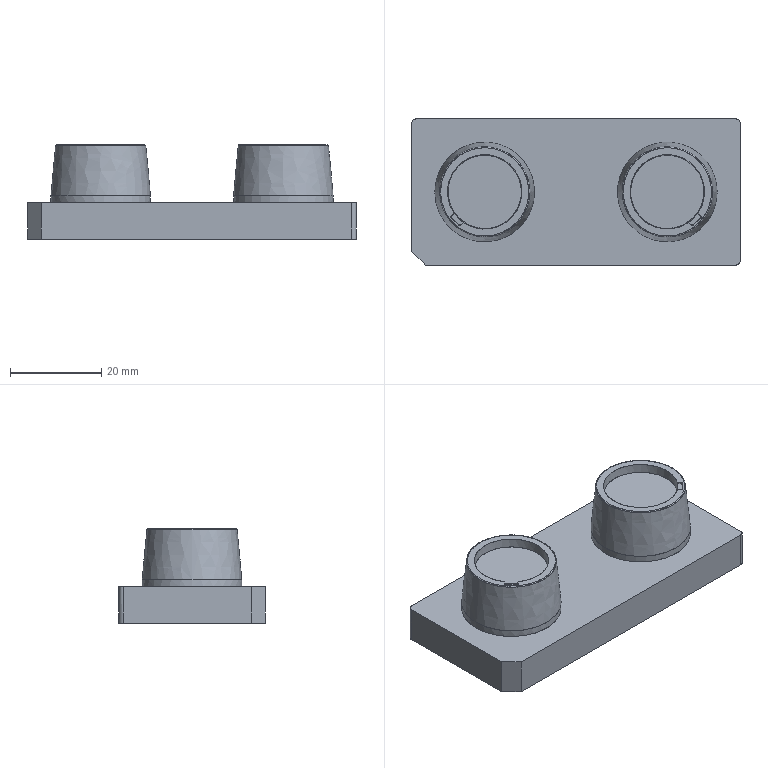NC program | PowerMill | posted with a generic post | part box 72 x 32 x 20.655 mm
Lines 1 to 915 of 315359:
%
O0001
N104 ( POWERMILL CB  : 2026004.0)
N105 ( POST VER      : 2026.0.0.5161)
N106 ( OPTION FILE   : FANUC)
N107 ( OUTPUT WORKPLANE : WORLD)
N108 (  )
N109 ( TOOL LIST )
N110 (---------------------------------------)
N111 ( NO. | ID        | DIA.| TIP RAD|LENGTH)
N112 (---------------------------------------)
N113 (    1|D10C_1_1_1 |10.0 |  0.0   |76.12 )
N114 (    2|D4C_1_1    | 4.0 |  0.0   |67.84 )
N115 (    3|D10_1_1_1  |10.0 |  0.0   | 75.8 )
N116 (    5|B4R0.5_1_1 | 4.0 |  0.5   | 67.8 )
N117 (    8|D1_1       | 1.0 |  0.0   | 56.0 )
N118 (   13|TEXT_D4_1_1| 4.0 |  0.3   |67.92 )
N119 (---------------------------------------)
N120 (  )
N121 ( NUMBER OF TOOLPATHS: 13.0 )
N122 ( ESTIMATED PROGRAM DURATION: 0 HOURS 36 MIN 15 SEC)
N123 (  )
N124 G00 G21 G80 G40 G17
N125 G90
N126 G54
N127 G53 Z0.0
N128 (---------------)
N129 ( START TOOLPATH : 精公开粗01-扫面平行-D10C )
N130 (---------------)
N131 ( TOOL NO.    :1 )
N132 ( TOOL TYPE   : ENDMILL)
N133 ( TOOL ID     : D10C_1_1_1)
N134 ( TOOL DIA    : 10.0 LENGTH 76.12)
N135 T1
N136 M6
N137 S8000 M03
N138 G00 G90 X0.0 Y0.0
N139 G43 Z10.2 H1
N140
N141 G05 P10000 R4
N142 X43.78 Y18.78
N143 Z1.135
N144 G01 Z-0.065 F6000.0
N145 X38.78 F10000.0
N146 X-38.78
N147 Y13.4143
N148 X38.78
N149 Y8.0486
N150 X-38.78
N151 Y2.6829
N152 X38.78
N153 Y-2.6829
N154 X-38.78
N155 Y-8.0486
N156 X38.78
N157 Y-13.4143
N158 X-38.78
N159 Y-18.78
N160 X38.78
N161 X43.78
N162 G00 Z10.2
N163 G05 P0
N164 (---------------)
N165 ( END TOOLPATH : 精公开粗01-扫面平行-D10C )
N166 (---------------)
N167 ( START TOOLPATH : 精公开粗01-外形偏置-D10C )
N168 (---------------)
N169 G00 X0.0 Y0.0 Z9.885
N170 G05 P10000 R4
N171 X19.903 Y-2.8285
N172 Z1.1899
N173 G01 Z-0.0101 F6000.0
N174 X20.1091 Y-2.8335 Z-0.0137
N175 X20.501 Y-2.7901 Z-0.0206
N176 X20.8825 Y-2.6933 Z-0.0274
N177 X21.2741 Y-2.5346 Z-0.0348
N178 X21.6402 Y-2.3203 Z-0.0422
N179 X21.9587 Y-2.1244 Z-0.0488
N180 X22.123 Y-1.96 Z-0.0528
N181 X22.4294 Y-1.4606 Z-0.063
N182 X22.6008 Y-1.1271 Z-0.0696
N183 X22.7288 Y-0.7734 Z-0.0761
N184 X22.8112 Y-0.3909 Z-0.083
N185 X22.835 Y0.0 Z-0.0898
N186 X22.8067 Y0.3906 Z-0.0966
N187 X22.726 Y0.7734 Z-0.1035
N188 X22.6003 Y1.1275 Z-0.11
N189 X22.4294 Y1.4635 Z-0.1166
N190 X22.2257 Y1.76 Z-0.1229
N191 X22.0503 Y1.9572 Z-0.1275
N192 X21.6237 Y2.3203 Z-0.1373
N193 X21.2669 Y2.5338 Z-0.1445
N194 X20.8825 Y2.695 Z-0.1518
N195 X20.5011 Y2.791 Z-0.1587
N196 X20.1091 Y2.8316 Z-0.1655
N197 X19.7195 Y2.8187 Z-0.1723
N198 X19.3357 Y2.7535 Z-0.1791
N199 X18.9368 Y2.6276 Z-0.1864
N200 X18.5622 Y2.4457 Z-0.1937
N201 X18.3116 Y2.2576 Z-0.1992
N202 X18.061 Y2.0696 Z-0.2046
N203 X17.9212 Y1.9247 Z-0.2081
N204 X17.6227 Y1.5469 Z-0.2166
N205 X17.4192 Y1.1743 Z-0.224
N206 X17.2744 Y0.7734 Z-0.2314
N207 X17.1936 Y0.3907 Z-0.2382
N208 X17.1655 Y0.0 Z-0.2451
N209 X17.1902 Y-0.3908 Z-0.2519
N210 X17.27 Y-0.7734 Z-0.2587
N211 X17.4201 Y-1.1736 Z-0.2662
N212 X17.6254 Y-1.5469 Z-0.2736
N213 X17.7888 Y-1.7726 Z-0.2785
N214 X18.0606 Y-2.0667 Z-0.2855
N215 X18.3701 Y-2.3203 Z-0.2924
N216 X18.5622 Y-2.4423 Z-0.2964
N217 X18.9369 Y-2.6281 Z-0.3037
N218 X19.3357 Y-2.7581 Z-0.311
N219 X19.7193 Y-2.824 Z-0.3178
N220 X20.1091 Y-2.8335 Z-0.3246
N221 X20.501 Y-2.7901 Z-0.3315
N222 X20.8825 Y-2.6933 Z-0.3384
N223 X21.2741 Y-2.5346 Z-0.3458
N224 X21.6402 Y-2.3203 Z-0.3532
N225 X21.9587 Y-2.1244 Z-0.3597
N226 X22.123 Y-1.96 Z-0.3637
N227 X22.4294 Y-1.4606 Z-0.374
N228 X22.6008 Y-1.1271 Z-0.3805
N229 X22.7288 Y-0.7734 Z-0.3871
N230 X22.8112 Y-0.3909 Z-0.3939
N231 X22.835 Y0.0 Z-0.4007
N232 X22.8067 Y0.3906 Z-0.4076
N233 X22.726 Y0.7734 Z-0.4144
N234 X22.6003 Y1.1275 Z-0.421
N235 X22.4294 Y1.4635 Z-0.4275
N236 X22.2257 Y1.76 Z-0.4338
N237 X22.0503 Y1.9572 Z-0.4384
N238 X21.6237 Y2.3203 Z-0.4482
N239 X21.2669 Y2.5338 Z-0.4555
N240 X20.8825 Y2.695 Z-0.4627
N241 X20.5011 Y2.791 Z-0.4696
N242 X20.1091 Y2.8316 Z-0.4765
N243 X19.7195 Y2.8187 Z-0.4833
N244 X19.3357 Y2.7535 Z-0.4901
N245 X18.9368 Y2.6276 Z-0.4974
N246 X18.5622 Y2.4457 Z-0.5046
N247 X18.3116 Y2.2576 Z-0.5101
N248 X18.061 Y2.0696 F10000.0
N249 X17.9212 Y1.9247
N250 X17.6227 Y1.5469
N251 X17.4192 Y1.1743
N252 X17.2744 Y0.7734
N253 X17.1936 Y0.3907
N254 X17.1655 Y0.0
N255 X17.1902 Y-0.3908
N256 X17.27 Y-0.7734
N257 X17.4201 Y-1.1736
N258 X17.6254 Y-1.5469
N259 X17.7888 Y-1.7726
N260 X18.0606 Y-2.0667
N261 X18.3701 Y-2.3203
N262 X18.5622 Y-2.4423
N263 X18.9369 Y-2.6281
N264 X19.3357 Y-2.7581
N265 X19.7193 Y-2.824
N266 X20.1091 Y-2.8335
N267 X20.501 Y-2.7901
N268 X20.8825 Y-2.6933
N269 X21.2741 Y-2.5346
N270 X21.6402 Y-2.3203
N271 X21.9587 Y-2.1244
N272 X22.0505 Y-2.0518
N273 X22.123 Y-1.96
N274 X22.4294 Y-1.4606
N275 X22.6008 Y-1.1271
N276 X22.7288 Y-0.7734
N277 X22.8112 Y-0.3909
N278 X22.835 Y0.0
N279 X22.8067 Y0.3906
N280 X22.726 Y0.7734
N281 X22.6003 Y1.1275
N282 X22.4294 Y1.4635
N283 X22.2257 Y1.76
N284 X22.0503 Y1.9572
N285 X21.6237 Y2.3203
N286 X21.2669 Y2.5338
N287 X20.8825 Y2.695
N288 X20.5011 Y2.791
N289 X20.1091 Y2.8316
N290 X19.7195 Y2.8187
N291 X19.3357 Y2.7535
N292 X18.9368 Y2.6276
N293 X18.5622 Y2.4457
N294 X18.3116 Y2.2576
N295 G00 Z5.843
N296 G01 X19.6442 Y-2.7896
N297 G00 Z-0.4052
N298 G01 X19.7191 Y-2.8028 Z-0.4065 F6000.0
N299 X20.1091 Y-2.8122 Z-0.4133
N300 X20.6953 Y-2.7282 Z-0.4237
N301 X21.251 Y-2.5191 Z-0.434
N302 X21.5966 Y-2.3203 Z-0.441
N303 X22.009 Y-1.9677 Z-0.4505
N304 X22.352 Y-1.5469 Z-0.4599
N305 X22.5869 Y-1.106 Z-0.4687
N306 X22.7066 Y-0.7734 Z-0.4748
N307 X22.7887 Y-0.3907 Z-0.4816
N308 X22.814 Y0.0 Z-0.4885
N309 X22.7858 Y0.3907 Z-0.4953
N310 X22.7044 Y0.7734 Z-0.5021
N311 X22.5869 Y1.1047 Z-0.5083
N312 X22.4294 Y1.4201 Z-0.5144
N313 X22.0357 Y1.9425 Z-0.5259
N314 X21.6559 Y2.2728 Z-0.5346
N315 X21.2477 Y2.5206 Z-0.543
N316 X20.8825 Y2.6728 Z-0.5499
N317 X20.5012 Y2.7702 Z-0.5567
N318 X20.1091 Y2.8113 Z-0.5636
N319 X19.7195 Y2.7979 Z-0.5704
N320 X19.3357 Y2.7321 Z-0.5772
N321 X18.9367 Y2.6046 Z-0.5845
N322 X18.5622 Y2.4207 Z-0.5918
N323 X18.3242 Y2.241 Z-0.597
N324 X18.0773 Y2.0546 Z-0.6024
N325 X17.9275 Y1.901 Z-0.6062
N326 X17.6489 Y1.5469 Z-0.614
N327 X17.4419 Y1.1751 Z-0.6214
N328 X17.2632 Y0.6374 Z-0.6313
N329 X17.2403 Y0.5302 Z-0.6333
N330 X17.1865 Y0.0 Z-0.6426
N331 X17.213 Y-0.3905 Z-0.6494
N332 X17.2921 Y-0.7734 Z-0.6562
N333 X17.4432 Y-1.174 Z-0.6637
N334 X17.6503 Y-1.5469 Z-0.6711
N335 X17.9254 Y-1.9026 Z-0.679
N336 X18.4084 Y-2.3203 Z-0.6901
N337 X18.7437 Y-2.5205 Z-0.6969
N338 X19.3357 Y-2.7349 Z-0.7079
N339 X19.7191 Y-2.8028 Z-0.7147
N340 X20.1091 Y-2.8122 Z-0.7215
N341 X20.6953 Y-2.7282 Z-0.7319
N342 X21.251 Y-2.5191 Z-0.7422
N343 X21.5966 Y-2.3203 Z-0.7492
N344 X22.009 Y-1.9677 Z-0.7586
N345 X22.352 Y-1.5469 Z-0.7681
N346 X22.5869 Y-1.106 Z-0.7768
N347 X22.7066 Y-0.7734 Z-0.783
N348 X22.7887 Y-0.3907 Z-0.7898
N349 X22.814 Y0.0 Z-0.7967
N350 X22.7858 Y0.3907 Z-0.8035
N351 X22.7044 Y0.7734 Z-0.8103
N352 X22.5869 Y1.1047 Z-0.8165
N353 X22.4294 Y1.4201 Z-0.8226
N354 X22.0357 Y1.9425 Z-0.834
N355 X21.6559 Y2.2728 Z-0.8428
N356 X21.2477 Y2.5206 Z-0.8512
N357 X20.8825 Y2.6728 Z-0.8581
N358 X20.5012 Y2.7702 Z-0.8649
N359 X20.1091 Y2.8113 Z-0.8718
N360 X19.7195 Y2.7979 Z-0.8786
N361 X19.3357 Y2.7321 Z-0.8854
N362 X18.9367 Y2.6046 Z-0.8927
N363 X18.5622 Y2.4207 Z-0.9
N364 X18.3242 Y2.241 Z-0.9052
N365 X18.0773 Y2.0546 F10000.0
N366 X17.9275 Y1.901
N367 X17.6489 Y1.5469
N368 X17.4419 Y1.1751
N369 X17.2632 Y0.6374
N370 X17.2488 Y0.5844
N371 X17.2403 Y0.5302
N372 X17.1865 Y0.0
N373 X17.213 Y-0.3905
N374 X17.2921 Y-0.7734
N375 X17.4432 Y-1.174
N376 X17.6503 Y-1.5469
N377 X17.9254 Y-1.9026
N378 X18.4084 Y-2.3203
N379 X18.7437 Y-2.5205
N380 X19.3357 Y-2.7349
N381 X19.7191 Y-2.8028
N382 X20.1091 Y-2.8122
N383 X20.6953 Y-2.7282
N384 X21.251 Y-2.5191
N385 X21.5966 Y-2.3203
N386 X22.009 Y-1.9677
N387 X22.352 Y-1.5469
N388 X22.5869 Y-1.106
N389 X22.7066 Y-0.7734
N390 X22.7887 Y-0.3907
N391 X22.814 Y0.0
N392 X22.7858 Y0.3907
N393 X22.7044 Y0.7734
N394 X22.5869 Y1.1047
N395 X22.4294 Y1.4201
N396 X22.0357 Y1.9425
N397 X21.6559 Y2.2728
N398 X21.2477 Y2.5206
N399 X20.8825 Y2.6728
N400 X20.5012 Y2.7702
N401 X20.1091 Y2.8113
N402 X19.7195 Y2.7979
N403 X19.3357 Y2.7321
N404 X18.9367 Y2.6046
N405 X18.5622 Y2.4207
N406 X18.3242 Y2.241
N407 G00 Z5.8378
N408 G01 X19.4393 Y-2.7343
N409 G00 Z-0.8003
N410 G01 X19.7204 Y-2.782 Z-0.8053 F6000.0
N411 X20.1091 Y-2.7908 Z-0.8121
N412 X20.5009 Y-2.7455 Z-0.8189
N413 X20.8825 Y-2.6474 Z-0.8258
N414 X21.2287 Y-2.5062 Z-0.8323
N415 X21.2573 Y-2.4898 Z-0.8329
N416 X21.5538 Y-2.3203 Z-0.8389
N417 X22.0217 Y-1.9256 Z-0.8496
N418 X22.3257 Y-1.5469 Z-0.858
N419 X22.5755 Y-1.0858 Z-0.8672
N420 X22.6843 Y-0.7734 Z-0.873
N421 X22.7692 Y-0.3911 Z-0.8798
N422 X22.7931 Y0.0 Z-0.8866
N423 X22.7639 Y0.3906 Z-0.8935
N424 X22.6828 Y0.7734 Z-0.9003
N425 X22.5737 Y1.0817 Z-0.906
N426 X22.3252 Y1.5469 Z-0.9152
N427 X22.0211 Y1.9278 Z-0.9237
N428 X21.6559 Y2.2476 Z-0.9322
N429 X21.2283 Y2.5071 Z-0.9409
N430 X20.8825 Y2.6506 Z-0.9475
N431 X20.5012 Y2.7493 Z-0.9543
N432 X20.1091 Y2.791 Z-0.9612
N433 X19.7195 Y2.7765 Z-0.968
N434 X19.3357 Y2.7107 Z-0.9748
N435 X18.9355 Y2.5843 Z-0.9821
N436 X18.5622 Y2.3957 Z-0.9894
N437 X18.3364 Y2.2248 Z-0.9944
N438 X18.0927 Y2.0405 Z-0.9997
N439 X17.6723 Y1.5469 Z-1.011
N440 X17.4644 Y1.175 Z-1.0185
N441 X17.3181 Y0.7734 Z-1.0259
N442 X17.2366 Y0.391 Z-1.0327
N443 X17.207 Y0.0 Z-1.0396
N444 X17.2308 Y-0.3908 Z-1.0464
N445 X17.3141 Y-0.7734 Z-1.0532
N446 X17.4676 Y-1.173 Z-1.0607
N447 X17.6756 Y-1.5469 Z-1.0682
N448 X17.7888 Y-1.7051 Z-1.0716
N449 X18.0926 Y-2.0376 Z-1.0794
N450 X18.4434 Y-2.3203 Z-1.0873
N451 X18.9388 Y-2.5811 Z-1.0971
N452 X19.3357 Y-2.7167 Z-1.1044
N453 X19.7204 Y-2.782 Z-1.1112
N454 X20.1091 Y-2.7908 Z-1.118
N455 X20.5009 Y-2.7455 Z-1.1249
N456 X20.8825 Y-2.6474 Z-1.1317
N457 X21.2287 Y-2.5062 Z-1.1383
N458 X21.2573 Y-2.4898 Z-1.1388
N459 X21.5538 Y-2.3203 Z-1.1448
N460 X22.0217 Y-1.9256 Z-1.1555
N461 X22.3257 Y-1.5469 Z-1.164
N462 X22.5755 Y-1.0858 Z-1.1731
N463 X22.6843 Y-0.7734 Z-1.1789
N464 X22.7692 Y-0.3911 Z-1.1857
N465 X22.7931 Y0.0 Z-1.1926
N466 X22.7639 Y0.3906 Z-1.1994
N467 X22.6828 Y0.7734 Z-1.2062
N468 X22.5737 Y1.0817 Z-1.2119
N469 X22.3252 Y1.5469 Z-1.2211
N470 X22.0211 Y1.9278 Z-1.2296
N471 X21.6559 Y2.2476 Z-1.2381
N472 X21.2283 Y2.5071 Z-1.2468
N473 X20.8825 Y2.6506 Z-1.2534
N474 X20.5012 Y2.7493 Z-1.2603
N475 X20.1091 Y2.791 Z-1.2671
N476 X19.7195 Y2.7765 Z-1.2739
N477 X19.3357 Y2.7107 Z-1.2807
N478 X18.9355 Y2.5843 Z-1.2881
N479 X18.5622 Y2.3957 Z-1.2954
N480 X18.3364 Y2.2248 Z-1.3003
N481 X18.0927 Y2.0405 F10000.0
N482 X17.6723 Y1.5469
N483 X17.4644 Y1.175
N484 X17.3181 Y0.7734
N485 X17.2366 Y0.391
N486 X17.207 Y0.0
N487 X17.2308 Y-0.3908
N488 X17.3141 Y-0.7734
N489 X17.4676 Y-1.173
N490 X17.6756 Y-1.5469
N491 X17.7888 Y-1.7051
N492 X18.0926 Y-2.0376
N493 X18.4434 Y-2.3203
N494 X18.9388 Y-2.5811
N495 X19.3357 Y-2.7167
N496 X19.7204 Y-2.782
N497 X20.1091 Y-2.7908
N498 X20.5009 Y-2.7455
N499 X20.8825 Y-2.6474
N500 X21.2287 Y-2.5062
N501 X21.2573 Y-2.4898
N502 X21.5538 Y-2.3203
N503 X22.0217 Y-1.9256
N504 X22.3257 Y-1.5469
N505 X22.5755 Y-1.0858
N506 X22.6843 Y-0.7734
N507 X22.7692 Y-0.3911
N508 X22.7931 Y0.0
N509 X22.7639 Y0.3906
N510 X22.6828 Y0.7734
N511 X22.5737 Y1.0817
N512 X22.3252 Y1.5469
N513 X22.0211 Y1.9278
N514 X21.6559 Y2.2476
N515 X21.2283 Y2.5071
N516 X20.8825 Y2.6506
N517 X20.5012 Y2.7493
N518 X20.1091 Y2.791
N519 X19.7195 Y2.7765
N520 X19.3357 Y2.7107
N521 X18.9355 Y2.5843
N522 X18.5622 Y2.3957
N523 X18.3364 Y2.2248
N524 G00 Z5.8314
N525 G01 X19.242 Y-2.6627
N526 G00 Z-1.1954
N527 G01 X19.3357 Y-2.6979 Z-1.1971 F6000.0
N528 X19.7205 Y-2.7602 Z-1.2039
N529 X20.1091 Y-2.772 Z-1.2107
N530 X20.6952 Y-2.6865 Z-1.2211
N531 X21.2078 Y-2.4931 Z-1.2306
N532 X21.5144 Y-2.3203 Z-1.2368
N533 X21.8394 Y-2.0772 Z-1.2439
N534 X22.1651 Y-1.7346 Z-1.2521
N535 X22.4294 Y-1.3385 Z-1.2604
N536 X22.6212 Y-0.9201 Z-1.2684
N537 X22.7482 Y-0.3904 Z-1.278
N538 X22.7675 Y-0.1944 Z-1.2814
N539 X22.743 Y0.3906 Z-1.2916
N540 X22.6612 Y0.7734 Z-1.2984
N541 X22.5597 Y1.0609 Z-1.3038
N542 X22.3001 Y1.5469 Z-1.3134
N543 X22.0064 Y1.913 Z-1.3216
N544 X21.6559 Y2.2224 Z-1.3297
N545 X21.209 Y2.4939 Z-1.3389
N546 X20.8825 Y2.6283 Z-1.345
N547 X20.5013 Y2.7289 Z-1.3519
N548 X19.9146 Y2.7721 Z-1.3622
N549 X19.3357 Y2.6893 Z-1.3724
N550 X18.935 Y2.5621 Z-1.3797
N551 X18.5622 Y2.3707 Z-1.387
N552 X18.3485 Y2.2088 Z-1.3917
N553 X18.1095 Y2.0277 Z-1.3969
N554 X17.7888 Y1.6748 Z-1.4053
N555 X17.4863 Y1.1741 Z-1.4155
N556 X17.3041 Y0.6376 Z-1.4253
N557 X17.2802 Y0.5291 Z-1.4273
N558 X17.2247 Y0.0 Z-1.4366
N559 X17.2505 Y-0.3906 Z-1.4434
N560 X17.3871 Y-0.9221 Z-1.453
N561 X17.4267 Y-1.0262 Z-1.4549
N562 X17.6677 Y-1.4953 Z-1.4641
N563 X17.7317 Y-1.5909 Z-1.4661
N564 X18.1036 Y-2.0278 Z-1.4762
N565 X18.4779 Y-2.3203 Z-1.4844
N566 X18.7449 Y-2.4761 Z-1.4898
N567 X19.3357 Y-2.6979 Z-1.5008
N568 X19.7205 Y-2.7602 Z-1.5077
N569 X20.1091 Y-2.772 Z-1.5144
N570 X20.6952 Y-2.6865 Z-1.5248
N571 X21.2078 Y-2.4931 Z-1.5343
N572 X21.5144 Y-2.3203 Z-1.5405
N573 X21.8394 Y-2.0772 Z-1.5476
N574 X22.1651 Y-1.7346 Z-1.5558
N575 X22.4294 Y-1.3385 Z-1.5641
N576 X22.6212 Y-0.9201 Z-1.5722
N577 X22.7482 Y-0.3904 Z-1.5817
N578 X22.7675 Y-0.1944 Z-1.5851
N579 X22.743 Y0.3906 Z-1.5953
N580 X22.6612 Y0.7734 Z-1.6021
N581 X22.5597 Y1.0609 Z-1.6075
N582 X22.3001 Y1.5469 Z-1.6171
N583 X22.0064 Y1.913 Z-1.6253
N584 X21.6559 Y2.2224 Z-1.6334
N585 X21.209 Y2.4939 Z-1.6426
N586 X20.8825 Y2.6283 Z-1.6487
N587 X20.5013 Y2.7289 Z-1.6556
N588 X19.9146 Y2.7721 Z-1.6659
N589 X19.3357 Y2.6893 Z-1.6761
N590 X18.935 Y2.5621 Z-1.6834
N591 X18.5622 Y2.3707 Z-1.6907
N592 X18.3485 Y2.2088 Z-1.6954
N593 X18.1095 Y2.0277 F10000.0
N594 X17.7888 Y1.6748
N595 X17.4863 Y1.1741
N596 X17.3041 Y0.6376
N597 X17.2891 Y0.584
N598 X17.2802 Y0.5291
N599 X17.2247 Y0.0
N600 X17.2505 Y-0.3906
N601 X17.3871 Y-0.9221
N602 X17.404 Y-0.9753
N603 X17.4267 Y-1.0262
N604 X17.6677 Y-1.4953
N605 X17.697 Y-1.545
N606 X17.7317 Y-1.5909
N607 X18.1036 Y-2.0278
N608 X18.4779 Y-2.3203
N609 X18.7449 Y-2.4761
N610 X19.3357 Y-2.6979
N611 X19.7205 Y-2.7602
N612 X20.1091 Y-2.772
N613 X20.6952 Y-2.6865
N614 X21.2078 Y-2.4931
N615 X21.5144 Y-2.3203
N616 X21.8394 Y-2.0772
N617 X22.1651 Y-1.7346
N618 X22.4294 Y-1.3385
N619 X22.6212 Y-0.9201
N620 X22.7482 Y-0.3904
N621 X22.7675 Y-0.1944
N622 X22.743 Y0.3906
N623 X22.6612 Y0.7734
N624 X22.5597 Y1.0609
N625 X22.3001 Y1.5469
N626 X22.0064 Y1.913
N627 X21.6559 Y2.2224
N628 X21.209 Y2.4939
N629 X20.8825 Y2.6283
N630 X20.5013 Y2.7289
N631 X19.9146 Y2.7721
N632 X19.3357 Y2.6893
N633 X18.935 Y2.5621
N634 X18.5622 Y2.3707
N635 X18.3485 Y2.2088
N636 G00 Z5.8228
N637 G01 X19.0596 Y-2.5789
N638 G00 Z-1.5905
N639 G01 X19.3357 Y-2.6766 Z-1.5956 F6000.0
N640 X19.7189 Y-2.7394 Z-1.6024
N641 X20.1091 Y-2.7563 Z-1.6092
N642 X20.5005 Y-2.7141 Z-1.6161
N643 X20.8825 Y-2.6039 Z-1.623
N644 X21.187 Y-2.4799 Z-1.6288
N645 X21.4749 Y-2.3203 Z-1.6345
N646 X21.8324 Y-2.0564 Z-1.6422
N647 X22.1504 Y-1.7305 Z-1.6502
N648 X22.4958 Y-1.1735 Z-1.6616
N649 X22.6482 Y-0.7734 Z-1.6691
N650 X22.7411 Y-0.2497 Z-1.6784
N651 X22.7482 Y-0.1377 Z-1.6803
N652 X22.7221 Y0.3906 Z-1.6896
N653 X22.6397 Y0.7734 Z-1.6964
N654 X22.4294 Y1.2929 Z-1.7062
N655 X22.275 Y1.5469 Z-1.7114
N656 X21.9918 Y1.8984 Z-1.7193
N657 X21.6559 Y2.1972 Z-1.7271
N658 X21.1897 Y2.4808 Z-1.7366
N659 X20.8825 Y2.6061 Z-1.7424
N660 X20.5016 Y2.7093 Z-1.7493
N661 X20.1091 Y2.7505 Z-1.7562
N662 X19.7195 Y2.7349 Z-1.763
N663 X19.3357 Y2.668 Z-1.7698
N664 X18.9346 Y2.5399 Z-1.7771
N665 X18.5622 Y2.3456 Z-1.7845
N666 X18.3607 Y2.1927 Z-1.7889
N667 X18.1249 Y2.0137 Z-1.7941
N668 X17.7888 Y1.642 Z-1.8028
N669 X17.508 Y1.1743 Z-1.8123
N670 X17.3553 Y0.7734 Z-1.8198
N671 X17.2733 Y0.3904 Z-1.8266
N672 X17.2451 Y0.0 Z-1.8335
N673 X17.271 Y-0.3897 Z-1.8403
N674 X17.3513 Y-0.7734 Z-1.8471
N675 X17.5121 Y-1.1702 Z-1.8546
N676 X17.719 Y-1.5469 Z-1.8621
N677 X18.1182 Y-2.0142 Z-1.8728
N678 X18.5125 Y-2.3203 Z-1.8815
N679 X18.9405 Y-2.5369 Z-1.8899
N680 X19.3357 Y-2.6766 Z-1.8972
N681 X19.7189 Y-2.7394 Z-1.904
N682 X20.1091 Y-2.7563 Z-1.9108
N683 X20.5005 Y-2.7141 Z-1.9177
N684 X20.8825 Y-2.6039 Z-1.9246
N685 X21.187 Y-2.4799 Z-1.9304
N686 X21.4749 Y-2.3203 Z-1.9361
N687 X21.8324 Y-2.0564 Z-1.9439
N688 X22.1504 Y-1.7305 Z-1.9518
N689 X22.4958 Y-1.1735 Z-1.9632
N690 X22.6482 Y-0.7734 Z-1.9707
N691 X22.7411 Y-0.2497 Z-1.98
N692 X22.7482 Y-0.1377 Z-1.982
N693 X22.7221 Y0.3906 Z-1.9912
N694 X22.6397 Y0.7734 Z-1.998
N695 X22.4294 Y1.2929 Z-2.0078
N696 X22.275 Y1.5469 Z-2.013
N697 X21.9918 Y1.8984 Z-2.0209
N698 X21.6559 Y2.1972 Z-2.0287
N699 X21.1897 Y2.4808 Z-2.0382
N700 X20.8825 Y2.6061 Z-2.044
N701 X20.5016 Y2.7093 Z-2.0509
N702 X20.1091 Y2.7505 Z-2.0578
N703 X19.7195 Y2.7349 Z-2.0646
N704 X19.3357 Y2.668 Z-2.0714
N705 X18.9346 Y2.5399 Z-2.0788
N706 X18.5622 Y2.3456 Z-2.0861
N707 X18.3607 Y2.1927 Z-2.0905
N708 X18.1249 Y2.0137 F10000.0
N709 X17.7888 Y1.642
N710 X17.508 Y1.1743
N711 X17.3553 Y0.7734
N712 X17.2733 Y0.3904
N713 X17.2451 Y0.0
N714 X17.271 Y-0.3897
N715 X17.3513 Y-0.7734
N716 X17.5121 Y-1.1702
N717 X17.719 Y-1.5469
N718 X18.1182 Y-2.0142
N719 X18.5125 Y-2.3203
N720 X18.9405 Y-2.5369
N721 X19.3357 Y-2.6766
N722 X19.7189 Y-2.7394
N723 X20.1091 Y-2.7563
N724 X20.5005 Y-2.7141
N725 X20.8825 Y-2.6039
N726 X21.187 Y-2.4799
N727 X21.4749 Y-2.3203
N728 X21.8324 Y-2.0564
N729 X22.1504 Y-1.7305
N730 X22.4958 Y-1.1735
N731 X22.6482 Y-0.7734
N732 X22.7411 Y-0.2497
N733 X22.7478 Y-0.1939
N734 X22.7482 Y-0.1377
N735 X22.7221 Y0.3906
N736 X22.6397 Y0.7734
N737 X22.4294 Y1.2929
N738 X22.275 Y1.5469
N739 X21.9918 Y1.8984
N740 X21.6559 Y2.1972
N741 X21.1897 Y2.4808
N742 X20.8825 Y2.6061
N743 X20.5016 Y2.7093
N744 X20.1091 Y2.7505
N745 X19.7195 Y2.7349
N746 X19.3357 Y2.668
N747 X18.9346 Y2.5399
N748 X18.5622 Y2.3456
N749 X18.3607 Y2.1927
N750 G00 Z3.6899
N751 G01 X-14.1404 Y-24.055
N752 G00 Z0.6899
N753 G01 Z-0.5101 F6000.0
N754 Y-23.5275 F10000.0
N755 G03 X-18.8879 Y-18.78 I-4.7475 J0.0
N756 G01 X-37.78
N757 G02 X-38.78 Y-17.78 I0.0 J1.0
N758 G01 Y17.78
N759 G02 X-37.78 Y18.78 I1.0 J0.0
N760 G01 X18.8883
N761 X19.1423 Y15.1437
N762 X19.3357 Y15.1572
N763 X20.1091 Y15.1708
N764 X20.8825 Y15.1444
N765 X21.6559 Y15.0788
N766 X22.4294 Y14.9733
N767 X23.2028 Y14.8274
N768 X23.763 Y14.6951
N769 X24.7496 Y14.4081
N770 X25.5231 Y14.1304
N771 X26.0242 Y13.9217
N772 X27.0699 Y13.4229
N773 X27.569 Y13.1483
N774 X28.6168 Y12.4837
N775 X29.3902 Y11.9139
N776 X30.1636 Y11.2639
N777 X30.9371 Y10.5107
N778 X31.7105 Y9.645
N779 X32.4839 Y8.6164
N780 X33.0519 Y7.7343
N781 X33.4808 Y6.9608
N782 X34.0308 Y5.7677
N783 X34.4422 Y4.6406
N784 X34.8042 Y3.313
N785 X34.9908 Y2.3203
N786 X35.0911 Y1.5469
N787 X35.1516 Y0.7734
N788 X35.1719 Y0.0
N789 X35.1515 Y-0.7734
N790 X35.0911 Y-1.5469
N791 X34.9909 Y-2.3203
N792 X34.8042 Y-3.3132
N793 X34.4422 Y-4.6406
N794 X34.0308 Y-5.7677
N795 X33.4808 Y-6.9608
N796 X33.0519 Y-7.7343
N797 X32.5589 Y-8.5077
N798 X31.9979 Y-9.2811
N799 X31.36 Y-10.0545
N800 X30.6253 Y-10.828
N801 X29.7726 Y-11.6014
N802 X28.7743 Y-12.3748
N803 X27.8434 Y-12.9844
N804 X27.0699 Y-13.4229
N805 X26.2965 Y-13.8034
N806 X25.5231 Y-14.1304
N807 X24.7496 Y-14.4081
N808 X23.763 Y-14.6951
N809 X23.2028 Y-14.8275
N810 X22.4294 Y-14.9733
N811 X21.6559 Y-15.0788
N812 X20.8825 Y-15.1444
N813 X20.1091 Y-15.1708
N814 X19.3357 Y-15.1573
N815 X18.5622 Y-15.1032
N816 X17.7888 Y-15.0084
N817 X17.0154 Y-14.8732
N818 X16.242 Y-14.6964
N819 X15.4685 Y-14.4763
N820 X14.6951 Y-14.2111
N821 X13.9756 Y-13.9217
N822 X13.1483 Y-13.5355
N823 X12.3748 Y-13.1165
N824 X11.2258 Y-12.3748
N825 X10.2275 Y-11.6014
N826 X9.3743 Y-10.828
N827 X8.6398 Y-10.0545
N828 X7.7343 Y-8.929
N829 X6.9608 Y-7.7547
N830 X6.5192 Y-6.9608
N831 X6.1874 Y-6.2759
N832 X5.8289 Y-5.414
N833 X5.414 Y-4.1751
N834 X5.1497 Y-3.0937
N835 X5.0092 Y-2.3203
N836 X4.909 Y-1.5469
N837 X4.8483 Y-0.7734
N838 X4.8281 Y0.0
N839 X4.8483 Y0.7734
N840 X4.909 Y1.5469
N841 X5.0092 Y2.3203
N842 X5.1497 Y3.0937
N843 X5.414 Y4.1747
N844 X5.8291 Y5.414
N845 X6.1479 Y6.1874
N846 X6.5192 Y6.9608
N847 X6.9483 Y7.7343
N848 X7.7343 Y8.9288
N849 X8.5077 Y9.9
N850 X9.2811 Y10.7371
N851 X10.2273 Y11.6014
N852 X11.2258 Y12.3748
N853 X12.3748 Y13.1165
N854 X13.1483 Y13.5355
N855 X13.9217 Y13.8987
N856 X14.6951 Y14.2112
N857 X15.4685 Y14.4763
N858 X16.237 Y14.6951
N859 X17.0154 Y14.8732
N860 X17.7888 Y15.0084
N861 X18.5622 Y15.1032
N862 X19.1423 Y15.1437
N863 X18.8883 Y18.78
N864 X37.78
N865 G02 X38.78 Y17.78 I0.0 J-1.0
N866 G01 Y-17.78
N867 G02 X37.78 Y-18.78 I-1.0 J0.0
N868 G01 X-1.2444
N869 X-1.2443 Y-13.4787
N870 G02 X-2.702 Y-11.0417 I0.0 J1.6544
N871 G01 X-1.8928 Y-9.5335
N872 X-1.2376 Y-8.2917
N873 G02 X1.2379 Y-8.2924 I1.2376 J-0.653
N874 G01 X2.6987 Y-11.0638
N875 G02 X1.2418 Y-13.4787 I-1.4569 J-0.768
N876 G01 X-1.2443
N877 X-1.2444 Y-18.78
N878 X-18.8879
N879 X-19.1423 Y-15.1437
N880 X-19.3357 Y-15.1573
N881 X-20.1091 Y-15.1708
N882 X-20.8825 Y-15.1444
N883 X-21.6559 Y-15.0788
N884 X-22.4294 Y-14.9733
N885 X-23.2028 Y-14.8275
N886 X-23.763 Y-14.6951
N887 X-24.7496 Y-14.4081
N888 X-25.5231 Y-14.1304
N889 X-26.0243 Y-13.9217
N890 X-27.0699 Y-13.4229
N891 X-27.5692 Y-13.1483
N892 X-28.6168 Y-12.4837
N893 X-29.3902 Y-11.9139
N894 X-30.1636 Y-11.2643
N895 X-30.9371 Y-10.5109
N896 X-31.7105 Y-9.645
N897 X-32.4839 Y-8.6165
N898 X-33.0516 Y-7.7343
N899 X-33.4808 Y-6.9608
N900 X-34.0308 Y-5.7677
N901 X-34.4421 Y-4.6406
N902 X-34.8042 Y-3.3132
N903 X-34.9908 Y-2.3203
N904 X-35.091 Y-1.5469
N905 X-35.1516 Y-0.7734
N906 X-35.1719 Y0.0
N907 X-35.1516 Y0.7734
N908 X-35.091 Y1.5469
N909 X-34.9909 Y2.3203
N910 X-34.8042 Y3.313
N911 X-34.4421 Y4.6406
N912 X-34.0308 Y5.7677
N913 X-33.4808 Y6.9608
N914 X-33.2573 Y7.3712
N915 X-32.5591 Y8.5077
N916 X-31.9979 Y9.2811
N917 X-31.3601 Y10.0545
N918 X-30.6257 Y10.828
N919 X-29.7726 Y11.6014
N920 X-28.7743 Y12.3748
N921 X-27.8434 Y12.9837
N922 X-27.0699 Y13.4229
N923 X-26.2965 Y13.8034
N924 X-25.5231 Y14.1304
N925 X-24.7496 Y14.4081
N926 X-23.9762 Y14.6398
N927 X-23.2028 Y14.8275
N928 X-22.4294 Y14.9733
N929 X-21.6559 Y15.0788
N930 X-20.8825 Y15.1444
N931 X-20.1091 Y15.1708
N932 X-19.3357 Y15.1572
N933 X-18.5622 Y15.1031
N934 X-17.7888 Y15.0084
N935 X-17.0154 Y14.8732
N936 X-16.242 Y14.6963
N937 X-15.4685 Y14.4763
N938 X-14.6951 Y14.2111
N939 X-13.9759 Y13.9217
N940 X-13.1483 Y13.5355
N941 X-12.3748 Y13.1165
N942 X-11.2258 Y12.3748
N943 X-10.2275 Y11.6014
N944 X-9.3746 Y10.828
N945 X-8.6398 Y10.0545
N946 X-7.7343 Y8.9289
N947 X-7.0269 Y7.855
N948 X-2.3357 Y10.3564
N949 X-2.7024 Y11.0442
N950 G02 X-1.2475 Y13.4787 I1.4549 J0.7825
N951 G01 X1.2377
N952 G02 X2.6945 Y11.0693 I0.0 J-1.6451
N953 G01 X1.2398 Y8.2963
N954 G02 X-1.2354 Y8.293 I-1.2385 J0.6498
N955 G01 X-2.3357 Y10.3564
N956 X-7.0269 Y7.855
N957 X-6.9608 Y7.7547
N958 X-6.5192 Y6.9608
N959 X-6.1874 Y6.2756
N960 X-5.8289 Y5.414
N961 X-5.414 Y4.1748
N962 X-5.1496 Y3.0937
N963 X-5.0092 Y2.3203
N964 X-4.9089 Y1.5469
N965 X-4.8484 Y0.7734
N966 X-4.8281 Y0.0
N967 X-4.8484 Y-0.7734
N968 X-4.9079 Y-1.5469
N969 X-5.0092 Y-2.3203
N970 X-5.1496 Y-3.0937
N971 X-5.414 Y-4.1751
N972 X-5.8291 Y-5.414
N973 X-6.1478 Y-6.1874
N974 X-6.5192 Y-6.9608
N975 X-6.9484 Y-7.7343
N976 X-7.7343 Y-8.929
N977 X-8.5077 Y-9.9
N978 X-9.2811 Y-10.7371
N979 X-10.2273 Y-11.6014
N980 X-11.2258 Y-12.3748
N981 X-12.3748 Y-13.1165
N982 X-13.1483 Y-13.5355
N983 X-13.9217 Y-13.8987
N984 X-14.6951 Y-14.2112
N985 X-15.4685 Y-14.4763
N986 X-16.237 Y-14.6951
N987 X-17.0154 Y-14.8732
N988 X-17.7888 Y-15.0084
N989 X-18.5622 Y-15.1031
N990 X-19.1423 Y-15.1437
N991 X-18.8879 Y-18.78
N992 G00 Z3.2948
N993 G01 X-14.1404 Y-24.055
N994 G00 Z0.2948
N995 G01 Z-0.9052 F6000.0
N996 Y-23.5275 F10000.0
N997 G03 X-18.8879 Y-18.78 I-4.7475 J0.0
N998 G01 X-37.78
N999 G02 X-38.78 Y-17.78 I0.0 J1.0
N1000 G01 Y-0.3847
N1001 X-35.2038 Y-0.29
N1002 X-35.2115 Y0.0
N1003 X-35.191 Y0.7734
N1004 X-35.1305 Y1.5469
N1005 X-35.0307 Y2.3203
N1006 X-34.8042 Y3.4931
N1007 X-34.4835 Y4.6406
N1008 X-34.0308 Y5.8697
N1009 X-33.5253 Y6.9608
N1010 X-33.2573 Y7.4526
N1011 X-32.6076 Y8.5077
N1012 X-32.048 Y9.2811